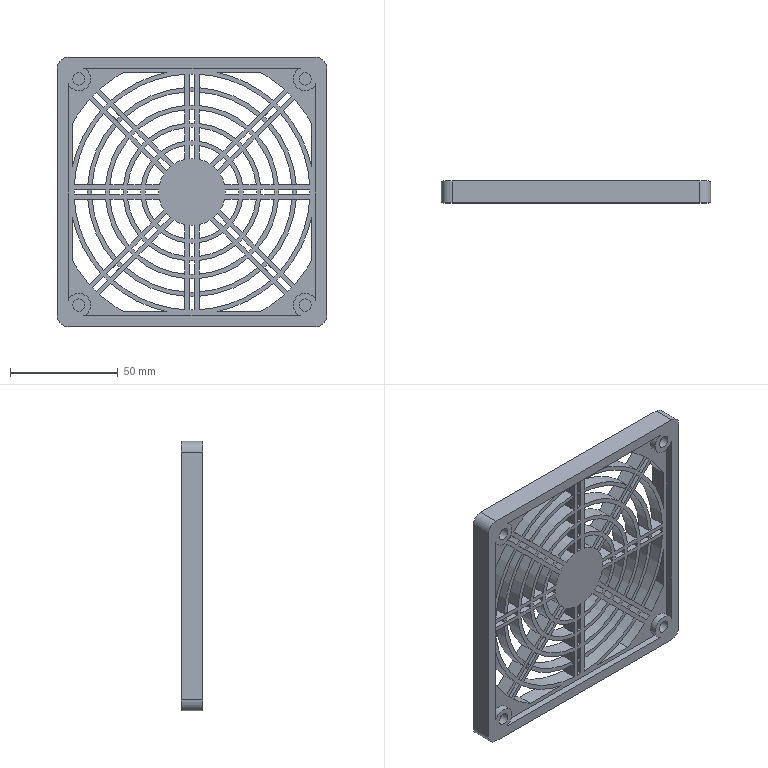Part | STEP file | E-PF-120-R | 1 solid | 379 faces | box 125 x 10 x 125 mm | volume 66671 mm3 | cylinder 196 | plane 183 | commonest cylinder face diameters 31 x16 43.5 x16 47.5 x16 60 x16 64 x16 76.5 x16